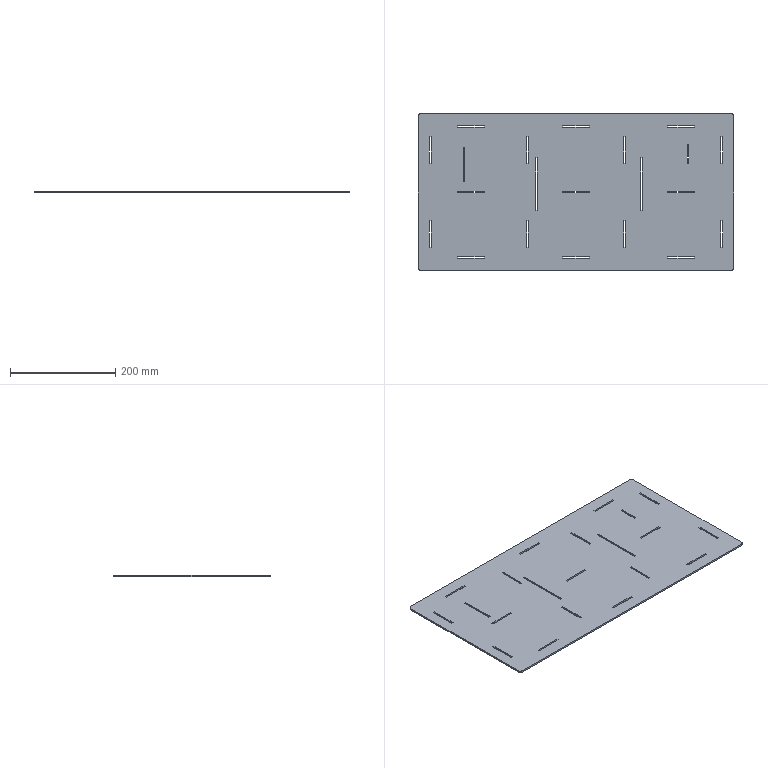Part | SolidWorks | features FlatPattern 1, SMBaseFlange 1, SheetMetal 1 | 1 solid | 94 faces | box 600 x 300 x 3.2 mm | volume 564155 mm3 | plane 90 | cylinder 4 | commonest cylinder face diameters 10 x4